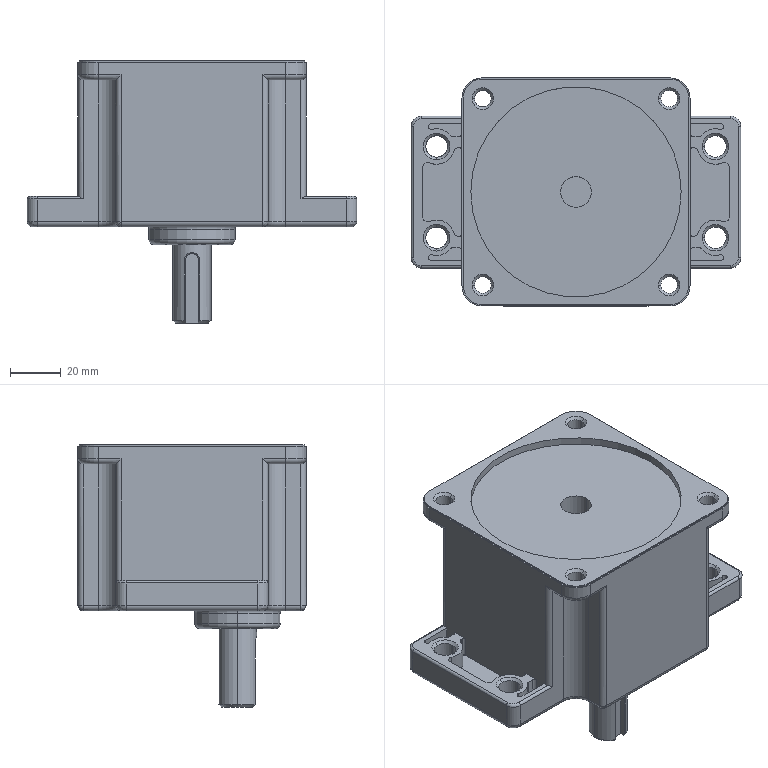Part | STEP file | S9KC75BH-S v20180123 (SPG Page91)-180713 | 1 solid | 239 faces | box 130 x 90 x 103.5 mm | volume 484588 mm3 | cylinder 112 | plane 61 | cone 35 | torus 20 | sphere 6 | spline 5 | commonest cylinder face diameters 4 x36 2 x26 14 x12 6.5 x8 8.5 x8 15 x6